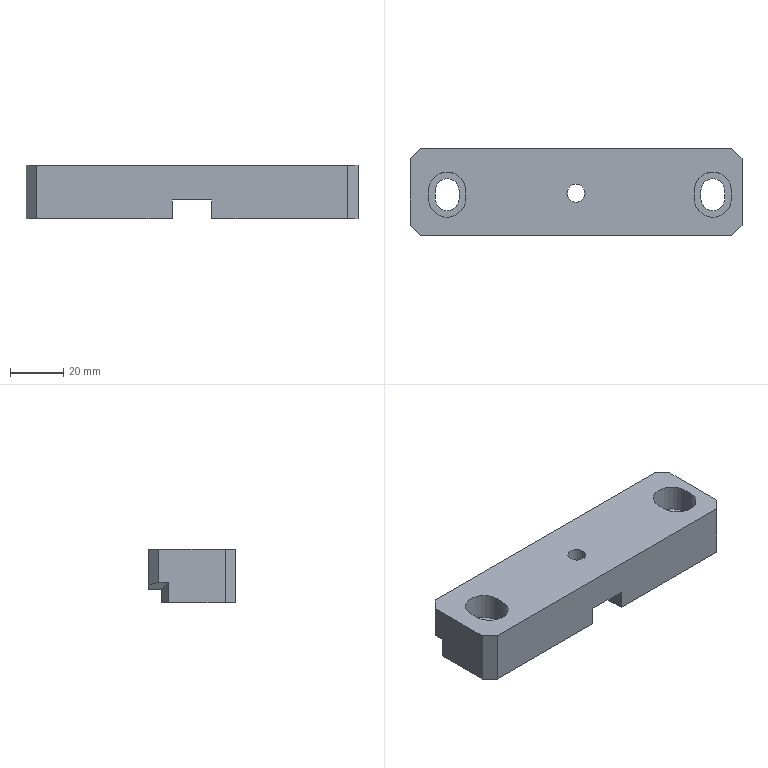Part | NX | features 20 2 | 1 solid | 41 faces | box 125 x 33 x 20 mm | volume 69243 mm3 | plane 32 | cylinder 9 | commonest cylinder face diameters 9 x4 14 x4 6.8 x1
STEP:
#1=CARTESIAN_POINT('',(3435.502,-433.5,16.5));
#2=VERTEX_POINT('',#1);
#3=CARTESIAN_POINT('',(3421.502,-433.5,16.5));
#4=VERTEX_POINT('',#3);
#5=CARTESIAN_POINT('',(3428.502,-433.5,16.5));
#6=DIRECTION('',(0.,0.,1.));
#7=DIRECTION('',(1.,0.,0.));
#8=AXIS2_PLACEMENT_3D('',#5,#6,#7);
#9=CIRCLE('',#8,7.);
#10=EDGE_CURVE('',#2,#4,#9,.T.);
#11=ORIENTED_EDGE('',*,*,#10,.F.);
#12=CARTESIAN_POINT('',(3435.502,-436.5,16.5));
#13=VERTEX_POINT('',#12);
#14=CARTESIAN_POINT('',(3435.502,-450.5,16.5));
#15=DIRECTION('',(0.,1.,0.));
#16=VECTOR('',#15,1000.);
#17=LINE('',#14,#16);
#18=EDGE_CURVE('',#13,#2,#17,.T.);
#19=ORIENTED_EDGE('',*,*,#18,.F.);
#20=CARTESIAN_POINT('',(3421.502,-436.5,16.5));
#21=VERTEX_POINT('',#20);
#22=CARTESIAN_POINT('',(3428.502,-436.5,16.5));
#23=DIRECTION('',(0.,0.,1.));
#24=DIRECTION('',(1.,0.,0.));
#25=AXIS2_PLACEMENT_3D('',#22,#23,#24);
#26=CIRCLE('',#25,7.);
#27=EDGE_CURVE('',#21,#13,#26,.T.);
#28=ORIENTED_EDGE('',*,*,#27,.F.);
#29=CARTESIAN_POINT('',(3421.502,-450.5,16.5));
#30=DIRECTION('',(0.,-1.,0.));
#31=VECTOR('',#30,1000.);
#32=LINE('',#29,#31);
#33=EDGE_CURVE('',#4,#21,#32,.T.);
#34=ORIENTED_EDGE('',*,*,#33,.F.);
#35=EDGE_LOOP('',(#11,#19,#28,#34));
#36=FACE_BOUND('',#35,.T.);
#37=CARTESIAN_POINT('',(3335.502,-436.5,16.5));
#38=VERTEX_POINT('',#37);
#39=CARTESIAN_POINT('',(3335.502,-433.5,16.5));
#40=VERTEX_POINT('',#39);
#41=CARTESIAN_POINT('',(3335.502,-450.5,16.5));
#42=DIRECTION('',(0.,1.,0.));
#43=VECTOR('',#42,1000.);
#44=LINE('',#41,#43);
#45=EDGE_CURVE('',#38,#40,#44,.T.);
#46=ORIENTED_EDGE('',*,*,#45,.F.);
#47=CARTESIAN_POINT('',(3321.502,-436.5,16.5));
#48=VERTEX_POINT('',#47);
#49=CARTESIAN_POINT('',(3328.502,-436.5,16.5));
#50=DIRECTION('',(0.,0.,1.));
#51=DIRECTION('',(1.,0.,0.));
#52=AXIS2_PLACEMENT_3D('',#49,#50,#51);
#53=CIRCLE('',#52,7.);
#54=EDGE_CURVE('',#48,#38,#53,.T.);
#55=ORIENTED_EDGE('',*,*,#54,.F.);
#56=CARTESIAN_POINT('',(3321.502,-433.5,16.5));
#57=VERTEX_POINT('',#56);
#58=CARTESIAN_POINT('',(3321.502,-450.5,16.5));
#59=DIRECTION('',(0.,-1.,0.));
#60=VECTOR('',#59,1000.);
#61=LINE('',#58,#60);
#62=EDGE_CURVE('',#57,#48,#61,.T.);
#63=ORIENTED_EDGE('',*,*,#62,.F.);
#64=CARTESIAN_POINT('',(3328.502,-433.5,16.5));
#65=DIRECTION('',(0.,0.,1.));
#66=DIRECTION('',(1.,0.,0.));
#67=AXIS2_PLACEMENT_3D('',#64,#65,#66);
#68=CIRCLE('',#67,7.);
#69=EDGE_CURVE('',#40,#57,#68,.T.);
#70=ORIENTED_EDGE('',*,*,#69,.F.);
#71=EDGE_LOOP('',(#46,#55,#63,#70));
#72=FACE_BOUND('',#71,.T.);
#73=CARTESIAN_POINT('',(3435.502,-417.5,16.5));
#74=VERTEX_POINT('',#73);
#75=CARTESIAN_POINT('',(3318.502,-417.5,16.5));
#76=VERTEX_POINT('',#75);
#77=CARTESIAN_POINT('',(3472.502,-417.5,16.5));
#78=DIRECTION('',(-1.,0.,0.));
#79=VECTOR('',#78,1000.);
#80=LINE('',#77,#79);
#81=EDGE_CURVE('',#74,#76,#80,.T.);
#82=ORIENTED_EDGE('',*,*,#81,.T.);
#83=CARTESIAN_POINT('',(3314.502,-421.5,16.5));
#84=VERTEX_POINT('',#83);
#85=CARTESIAN_POINT('',(3314.502,-421.5,16.5));
#86=DIRECTION('',(-0.7071,-0.7071,0.));
#87=VECTOR('',#86,1000.);
#88=LINE('',#85,#87);
#89=EDGE_CURVE('',#76,#84,#88,.T.);
#90=ORIENTED_EDGE('',*,*,#89,.T.);
#91=CARTESIAN_POINT('',(3314.502,-446.5,16.5));
#92=VERTEX_POINT('',#91);
#93=CARTESIAN_POINT('',(3314.502,-417.5,16.5));
#94=DIRECTION('',(0.,-1.,0.));
#95=VECTOR('',#94,1000.);
#96=LINE('',#93,#95);
#97=EDGE_CURVE('',#84,#92,#96,.T.);
#98=ORIENTED_EDGE('',*,*,#97,.T.);
#99=CARTESIAN_POINT('',(3318.502,-450.5,16.5));
#100=VERTEX_POINT('',#99);
#101=CARTESIAN_POINT('',(3318.502,-450.5,16.5));
#102=DIRECTION('',(0.7071,-0.7071,0.));
#103=VECTOR('',#102,1000.);
#104=LINE('',#101,#103);
#105=EDGE_CURVE('',#92,#100,#104,.T.);
#106=ORIENTED_EDGE('',*,*,#105,.T.);
#107=CARTESIAN_POINT('',(3435.502,-450.5,16.5));
#108=VERTEX_POINT('',#107);
#109=CARTESIAN_POINT('',(3392.502,-450.5,16.5));
#110=DIRECTION('',(1.,0.,0.));
#111=VECTOR('',#110,1000.);
#112=LINE('',#109,#111);
#113=EDGE_CURVE('',#100,#108,#112,.T.);
#114=ORIENTED_EDGE('',*,*,#113,.T.);
#115=CARTESIAN_POINT('',(3439.502,-446.5,16.5));
#116=VERTEX_POINT('',#115);
#117=CARTESIAN_POINT('',(3439.502,-446.5,16.5));
#118=DIRECTION('',(0.7071,0.7071,0.));
#119=VECTOR('',#118,1000.);
#120=LINE('',#117,#119);
#121=EDGE_CURVE('',#108,#116,#120,.T.);
#122=ORIENTED_EDGE('',*,*,#121,.T.);
#123=CARTESIAN_POINT('',(3439.502,-421.5,16.5));
#124=VERTEX_POINT('',#123);
#125=CARTESIAN_POINT('',(3439.502,-450.5,16.5));
#126=DIRECTION('',(0.,1.,0.));
#127=VECTOR('',#126,1000.);
#128=LINE('',#125,#127);
#129=EDGE_CURVE('',#116,#124,#128,.T.);
#130=ORIENTED_EDGE('',*,*,#129,.T.);
#131=CARTESIAN_POINT('',(3435.502,-417.5,16.5));
#132=DIRECTION('',(-0.7071,0.7071,0.));
#133=VECTOR('',#132,1000.);
#134=LINE('',#131,#133);
#135=EDGE_CURVE('',#124,#74,#134,.T.);
#136=ORIENTED_EDGE('',*,*,#135,.T.);
#137=EDGE_LOOP('',(#82,#90,#98,#106,#114,#122,#130,#136));
#138=FACE_BOUND('',#137,.T.);
#139=CARTESIAN_POINT('',(3380.402,-434.5,16.5));
#140=VERTEX_POINT('',#139);
#141=CARTESIAN_POINT('',(3377.002,-434.5,16.5));
#142=DIRECTION('',(0.,0.,-1.));
#143=DIRECTION('',(1.,0.,0.));
#144=AXIS2_PLACEMENT_3D('',#141,#142,#143);
#145=CIRCLE('',#144,3.4);
#146=EDGE_CURVE('',#140,#140,#145,.T.);
#147=ORIENTED_EDGE('',*,*,#146,.T.);
#148=EDGE_LOOP('',(#147));
#149=FACE_BOUND('',#148,.T.);
#150=CARTESIAN_POINT('',(3472.502,-450.5,16.5));
#151=DIRECTION('',(0.,0.,1.));
#152=DIRECTION('',(-1.,0.,0.));
#153=AXIS2_PLACEMENT_3D('',#150,#151,#152);
#154=PLANE('',#153);
#155=ADVANCED_FACE('',(#36,#72,#138,#149),#154,.T.);
#156=CARTESIAN_POINT('',(3384.502,-417.5,3.5));
#157=VERTEX_POINT('',#156);
#158=CARTESIAN_POINT('',(3384.502,-450.5,3.5));
#159=VERTEX_POINT('',#158);
#160=CARTESIAN_POINT('',(3384.502,-436.5,3.5));
#161=DIRECTION('',(0.,-1.,0.));
#162=VECTOR('',#161,1000.);
#163=LINE('',#160,#162);
#164=EDGE_CURVE('',#157,#159,#163,.T.);
#165=ORIENTED_EDGE('',*,*,#164,.F.);
#166=CARTESIAN_POINT('',(3384.502,-417.5,1.5));
#167=VERTEX_POINT('',#166);
#168=CARTESIAN_POINT('',(3384.502,-417.5,11.5));
#169=DIRECTION('',(0.,0.,-1.));
#170=VECTOR('',#169,1000.);
#171=LINE('',#168,#170);
#172=EDGE_CURVE('',#157,#167,#171,.T.);
#173=ORIENTED_EDGE('',*,*,#172,.T.);
#174=CARTESIAN_POINT('',(3384.502,-422.5,1.5));
#175=VERTEX_POINT('',#174);
#176=CARTESIAN_POINT('',(3384.502,-396.891,1.5));
#177=DIRECTION('',(0.,1.,0.));
#178=VECTOR('',#177,1000.);
#179=LINE('',#176,#178);
#180=EDGE_CURVE('',#175,#167,#179,.T.);
#181=ORIENTED_EDGE('',*,*,#180,.F.);
#182=CARTESIAN_POINT('',(3384.502,-422.5,-3.5));
#183=VERTEX_POINT('',#182);
#184=CARTESIAN_POINT('',(3384.502,-422.5,3.5));
#185=DIRECTION('',(0.,0.,-1.));
#186=VECTOR('',#185,1000.);
#187=LINE('',#184,#186);
#188=EDGE_CURVE('',#175,#183,#187,.T.);
#189=ORIENTED_EDGE('',*,*,#188,.T.);
#190=CARTESIAN_POINT('',(3384.502,-450.5,-3.5));
#191=VERTEX_POINT('',#190);
#192=CARTESIAN_POINT('',(3384.502,-450.5,-3.5));
#193=DIRECTION('',(0.,-1.,0.));
#194=VECTOR('',#193,1000.);
#195=LINE('',#192,#194);
#196=EDGE_CURVE('',#183,#191,#195,.T.);
#197=ORIENTED_EDGE('',*,*,#196,.T.);
#198=CARTESIAN_POINT('',(3384.502,-450.5,11.5));
#199=DIRECTION('',(0.,0.,1.));
#200=VECTOR('',#199,1000.);
#201=LINE('',#198,#200);
#202=EDGE_CURVE('',#191,#159,#201,.T.);
#203=ORIENTED_EDGE('',*,*,#202,.T.);
#204=EDGE_LOOP('',(#165,#173,#181,#189,#197,#203));
#205=FACE_BOUND('',#204,.T.);
#206=CARTESIAN_POINT('',(3384.502,-436.5,0.));
#207=DIRECTION('',(-1.,0.,0.));
#208=DIRECTION('',(0.,0.,1.));
#209=AXIS2_PLACEMENT_3D('',#206,#207,#208);
#210=PLANE('',#209);
#211=ADVANCED_FACE('',(#205),#210,.T.);
#212=CARTESIAN_POINT('',(3369.502,-422.5,-3.5));
#213=VERTEX_POINT('',#212);
#214=CARTESIAN_POINT('',(3369.502,-450.5,-3.5));
#215=VERTEX_POINT('',#214);
#216=CARTESIAN_POINT('',(3369.502,-450.5,-3.5));
#217=DIRECTION('',(0.,-1.,0.));
#218=VECTOR('',#217,1000.);
#219=LINE('',#216,#218);
#220=EDGE_CURVE('',#213,#215,#219,.T.);
#221=ORIENTED_EDGE('',*,*,#220,.F.);
#222=CARTESIAN_POINT('',(3369.502,-422.5,1.5));
#223=VERTEX_POINT('',#222);
#224=CARTESIAN_POINT('',(3369.502,-422.5,3.5));
#225=DIRECTION('',(0.,0.,-1.));
#226=VECTOR('',#225,1000.);
#227=LINE('',#224,#226);
#228=EDGE_CURVE('',#223,#213,#227,.T.);
#229=ORIENTED_EDGE('',*,*,#228,.F.);
#230=CARTESIAN_POINT('',(3369.502,-417.5,1.5));
#231=VERTEX_POINT('',#230);
#232=CARTESIAN_POINT('',(3369.502,-396.891,1.5));
#233=DIRECTION('',(0.,1.,0.));
#234=VECTOR('',#233,1000.);
#235=LINE('',#232,#234);
#236=EDGE_CURVE('',#223,#231,#235,.T.);
#237=ORIENTED_EDGE('',*,*,#236,.T.);
#238=CARTESIAN_POINT('',(3369.502,-417.5,3.5));
#239=VERTEX_POINT('',#238);
#240=CARTESIAN_POINT('',(3369.502,-417.5,11.5));
#241=DIRECTION('',(0.,0.,-1.));
#242=VECTOR('',#241,1000.);
#243=LINE('',#240,#242);
#244=EDGE_CURVE('',#239,#231,#243,.T.);
#245=ORIENTED_EDGE('',*,*,#244,.F.);
#246=CARTESIAN_POINT('',(3369.502,-450.5,3.5));
#247=VERTEX_POINT('',#246);
#248=CARTESIAN_POINT('',(3369.502,-436.5,3.5));
#249=DIRECTION('',(0.,1.,0.));
#250=VECTOR('',#249,1000.);
#251=LINE('',#248,#250);
#252=EDGE_CURVE('',#247,#239,#251,.T.);
#253=ORIENTED_EDGE('',*,*,#252,.F.);
#254=CARTESIAN_POINT('',(3369.502,-450.5,11.5));
#255=DIRECTION('',(0.,0.,1.));
#256=VECTOR('',#255,1000.);
#257=LINE('',#254,#256);
#258=EDGE_CURVE('',#215,#247,#257,.T.);
#259=ORIENTED_EDGE('',*,*,#258,.F.);
#260=EDGE_LOOP('',(#221,#229,#237,#245,#253,#259));
#261=FACE_BOUND('',#260,.T.);
#262=CARTESIAN_POINT('',(3369.502,-436.5,-9.5));
#263=DIRECTION('',(-1.,0.,0.));
#264=DIRECTION('',(0.,0.,-1.));
#265=AXIS2_PLACEMENT_3D('',#262,#263,#264);
#266=PLANE('',#265);
#267=ADVANCED_FACE('',(#261),#266,.F.);
#268=CARTESIAN_POINT('',(3380.402,-434.5,3.5));
#269=VERTEX_POINT('',#268);
#270=CARTESIAN_POINT('',(3377.002,-434.5,3.5));
#271=DIRECTION('',(0.,0.,1.));
#272=DIRECTION('',(1.,0.,0.));
#273=AXIS2_PLACEMENT_3D('',#270,#271,#272);
#274=CIRCLE('',#273,3.4);
#275=EDGE_CURVE('',#269,#269,#274,.T.);
#276=ORIENTED_EDGE('',*,*,#275,.T.);
#277=EDGE_LOOP('',(#276));
#278=FACE_BOUND('',#277,.T.);
#279=CARTESIAN_POINT('',(3447.502,-450.5,3.5));
#280=DIRECTION('',(1.,0.,0.));
#281=VECTOR('',#280,1000.);
#282=LINE('',#279,#281);
#283=EDGE_CURVE('',#247,#159,#282,.T.);
#284=ORIENTED_EDGE('',*,*,#283,.F.);
#285=ORIENTED_EDGE('',*,*,#252,.T.);
#286=CARTESIAN_POINT('',(3527.502,-417.5,3.5));
#287=DIRECTION('',(-1.,0.,0.));
#288=VECTOR('',#287,1000.);
#289=LINE('',#286,#288);
#290=EDGE_CURVE('',#157,#239,#289,.T.);
#291=ORIENTED_EDGE('',*,*,#290,.F.);
#292=ORIENTED_EDGE('',*,*,#164,.T.);
#293=EDGE_LOOP('',(#284,#285,#291,#292));
#294=FACE_BOUND('',#293,.T.);
#295=CARTESIAN_POINT('',(3377.002,-436.5,3.5));
#296=DIRECTION('',(0.,0.,1.));
#297=DIRECTION('',(0.,-1.,0.));
#298=AXIS2_PLACEMENT_3D('',#295,#296,#297);
#299=PLANE('',#298);
#300=ADVANCED_FACE('',(#278,#294),#299,.F.);
#301=CARTESIAN_POINT('',(3424.002,-436.5,6.5));
#302=VERTEX_POINT('',#301);
#303=CARTESIAN_POINT('',(3424.002,-433.5,6.5));
#304=VERTEX_POINT('',#303);
#305=CARTESIAN_POINT('',(3424.002,-432.5,6.5));
#306=DIRECTION('',(0.,1.,0.));
#307=VECTOR('',#306,1000.);
#308=LINE('',#305,#307);
#309=EDGE_CURVE('',#302,#304,#308,.T.);
#310=ORIENTED_EDGE('',*,*,#309,.T.);
#311=CARTESIAN_POINT('',(3433.002,-433.5,6.5));
#312=VERTEX_POINT('',#311);
#313=CARTESIAN_POINT('',(3428.502,-433.5,6.5));
#314=DIRECTION('',(0.,0.,-1.));
#315=DIRECTION('',(-1.,0.,0.));
#316=AXIS2_PLACEMENT_3D('',#313,#314,#315);
#317=CIRCLE('',#316,4.5);
#318=EDGE_CURVE('',#304,#312,#317,.T.);
#319=ORIENTED_EDGE('',*,*,#318,.T.);
#320=CARTESIAN_POINT('',(3433.002,-436.5,6.5));
#321=VERTEX_POINT('',#320);
#322=CARTESIAN_POINT('',(3433.002,-439.5,6.5));
#323=DIRECTION('',(0.,-1.,0.));
#324=VECTOR('',#323,1000.);
#325=LINE('',#322,#324);
#326=EDGE_CURVE('',#312,#321,#325,.T.);
#327=ORIENTED_EDGE('',*,*,#326,.T.);
#328=CARTESIAN_POINT('',(3428.502,-436.5,6.5));
#329=DIRECTION('',(0.,0.,-1.));
#330=DIRECTION('',(-1.,0.,0.));
#331=AXIS2_PLACEMENT_3D('',#328,#329,#330);
#332=CIRCLE('',#331,4.5);
#333=EDGE_CURVE('',#321,#302,#332,.T.);
#334=ORIENTED_EDGE('',*,*,#333,.T.);
#335=EDGE_LOOP('',(#310,#319,#327,#334));
#336=FACE_BOUND('',#335,.T.);
#337=CARTESIAN_POINT('',(3435.502,-433.5,6.5));
#338=VERTEX_POINT('',#337);
#339=CARTESIAN_POINT('',(3421.502,-433.5,6.5));
#340=VERTEX_POINT('',#339);
#341=CARTESIAN_POINT('',(3428.502,-433.5,6.5));
#342=DIRECTION('',(0.,0.,1.));
#343=DIRECTION('',(-1.,0.,0.));
#344=AXIS2_PLACEMENT_3D('',#341,#342,#343);
#345=CIRCLE('',#344,7.);
#346=EDGE_CURVE('',#338,#340,#345,.T.);
#347=ORIENTED_EDGE('',*,*,#346,.T.);
#348=CARTESIAN_POINT('',(3421.502,-436.5,6.5));
#349=VERTEX_POINT('',#348);
#350=CARTESIAN_POINT('',(3421.502,-439.5,6.5));
#351=DIRECTION('',(0.,-1.,0.));
#352=VECTOR('',#351,1000.);
#353=LINE('',#350,#352);
#354=EDGE_CURVE('',#340,#349,#353,.T.);
#355=ORIENTED_EDGE('',*,*,#354,.T.);
#356=CARTESIAN_POINT('',(3435.502,-436.5,6.5));
#357=VERTEX_POINT('',#356);
#358=CARTESIAN_POINT('',(3428.502,-436.5,6.5));
#359=DIRECTION('',(0.,0.,1.));
#360=DIRECTION('',(-1.,0.,0.));
#361=AXIS2_PLACEMENT_3D('',#358,#359,#360);
#362=CIRCLE('',#361,7.);
#363=EDGE_CURVE('',#349,#357,#362,.T.);
#364=ORIENTED_EDGE('',*,*,#363,.T.);
#365=CARTESIAN_POINT('',(3435.502,-432.5,6.5));
#366=DIRECTION('',(0.,1.,0.));
#367=VECTOR('',#366,1000.);
#368=LINE('',#365,#367);
#369=EDGE_CURVE('',#357,#338,#368,.T.);
#370=ORIENTED_EDGE('',*,*,#369,.T.);
#371=EDGE_LOOP('',(#347,#355,#364,#370));
#372=FACE_BOUND('',#371,.T.);
#373=CARTESIAN_POINT('',(3428.502,-432.5,6.5));
#374=DIRECTION('',(0.,0.,-1.));
#375=DIRECTION('',(1.,0.,0.));
#376=AXIS2_PLACEMENT_3D('',#373,#374,#375);
#377=PLANE('',#376);
#378=ADVANCED_FACE('',(#336,#372),#377,.F.);
#379=CARTESIAN_POINT('',(3429.502,-417.5,1.5));
#380=VERTEX_POINT('',#379);
#381=CARTESIAN_POINT('',(3429.502,-422.5,1.5));
#382=VERTEX_POINT('',#381);
#383=CARTESIAN_POINT('',(3429.502,-425.18,1.5));
#384=DIRECTION('',(0.,-1.,0.));
#385=VECTOR('',#384,1000.);
#386=LINE('',#383,#385);
#387=EDGE_CURVE('',#380,#382,#386,.T.);
#388=ORIENTED_EDGE('',*,*,#387,.F.);
#389=CARTESIAN_POINT('',(3435.502,-417.5,3.108));
#390=VERTEX_POINT('',#389);
#391=CARTESIAN_POINT('',(3429.502,-417.5,1.5));
#392=DIRECTION('',(-0.9659,0.,-0.2588));
#393=VECTOR('',#392,1000.);
#394=LINE('',#391,#393);
#395=EDGE_CURVE('',#390,#380,#394,.T.);
#396=ORIENTED_EDGE('',*,*,#395,.F.);
#397=CARTESIAN_POINT('',(3439.502,-421.5,4.179));
#398=VERTEX_POINT('',#397);
#399=CARTESIAN_POINT('',(3422.451,-404.449,-0.3894));
#400=DIRECTION('',(0.6947,-0.6947,0.1862));
#401=VECTOR('',#400,1000.);
#402=LINE('',#399,#401);
#403=EDGE_CURVE('',#390,#398,#402,.T.);
#404=ORIENTED_EDGE('',*,*,#403,.T.);
#405=CARTESIAN_POINT('',(3439.502,-425.18,4.179));
#406=VERTEX_POINT('',#405);
#407=CARTESIAN_POINT('',(3439.502,-417.5,4.179));
#408=DIRECTION('',(0.,1.,0.));
#409=VECTOR('',#408,1000.);
#410=LINE('',#407,#409);
#411=EDGE_CURVE('',#406,#398,#410,.T.);
#412=ORIENTED_EDGE('',*,*,#411,.F.);
#413=CARTESIAN_POINT('',(3438.875,-425.012,4.011));
#414=DIRECTION('',(0.9351,-0.2506,0.2506));
#415=VECTOR('',#414,1000.);
#416=LINE('',#413,#415);
#417=EDGE_CURVE('',#382,#406,#416,.T.);
#418=ORIENTED_EDGE('',*,*,#417,.F.);
#419=EDGE_LOOP('',(#388,#396,#404,#412,#418));
#420=FACE_BOUND('',#419,.T.);
#421=CARTESIAN_POINT('',(3429.502,-396.891,1.5));
#422=DIRECTION('',(0.2588,0.,-0.9659));
#423=DIRECTION('',(0.9659,0.,0.2588));
#424=AXIS2_PLACEMENT_3D('',#421,#422,#423);
#425=PLANE('',#424);
#426=ADVANCED_FACE('',(#420),#425,.T.);
#427=CARTESIAN_POINT('',(3333.002,-433.5,6.5));
#428=VERTEX_POINT('',#427);
#429=CARTESIAN_POINT('',(3333.002,-436.5,6.5));
#430=VERTEX_POINT('',#429);
#431=CARTESIAN_POINT('',(3333.002,-432.5,6.5));
#432=DIRECTION('',(0.,-1.,0.));
#433=VECTOR('',#432,1000.);
#434=LINE('',#431,#433);
#435=EDGE_CURVE('',#428,#430,#434,.T.);
#436=ORIENTED_EDGE('',*,*,#435,.T.);
#437=CARTESIAN_POINT('',(3324.002,-436.5,6.5));
#438=VERTEX_POINT('',#437);
#439=CARTESIAN_POINT('',(3328.502,-436.5,6.5));
#440=DIRECTION('',(0.,0.,-1.));
#441=DIRECTION('',(-1.,0.,0.));
#442=AXIS2_PLACEMENT_3D('',#439,#440,#441);
#443=CIRCLE('',#442,4.5);
#444=EDGE_CURVE('',#430,#438,#443,.T.);
#445=ORIENTED_EDGE('',*,*,#444,.T.);
#446=CARTESIAN_POINT('',(3324.002,-433.5,6.5));
#447=VERTEX_POINT('',#446);
#448=CARTESIAN_POINT('',(3324.002,-439.5,6.5));
#449=DIRECTION('',(0.,1.,0.));
#450=VECTOR('',#449,1000.);
#451=LINE('',#448,#450);
#452=EDGE_CURVE('',#438,#447,#451,.T.);
#453=ORIENTED_EDGE('',*,*,#452,.T.);
#454=CARTESIAN_POINT('',(3328.502,-433.5,6.5));
#455=DIRECTION('',(0.,0.,-1.));
#456=DIRECTION('',(-1.,0.,0.));
#457=AXIS2_PLACEMENT_3D('',#454,#455,#456);
#458=CIRCLE('',#457,4.5);
#459=EDGE_CURVE('',#447,#428,#458,.T.);
#460=ORIENTED_EDGE('',*,*,#459,.T.);
#461=EDGE_LOOP('',(#436,#445,#453,#460));
#462=FACE_BOUND('',#461,.T.);
#463=CARTESIAN_POINT('',(3335.502,-433.5,6.5));
#464=VERTEX_POINT('',#463);
#465=CARTESIAN_POINT('',(3321.502,-433.5,6.5));
#466=VERTEX_POINT('',#465);
#467=CARTESIAN_POINT('',(3328.502,-433.5,6.5));
#468=DIRECTION('',(0.,0.,1.));
#469=DIRECTION('',(-1.,0.,0.));
#470=AXIS2_PLACEMENT_3D('',#467,#468,#469);
#471=CIRCLE('',#470,7.);
#472=EDGE_CURVE('',#464,#466,#471,.T.);
#473=ORIENTED_EDGE('',*,*,#472,.T.);
#474=CARTESIAN_POINT('',(3321.502,-436.5,6.5));
#475=VERTEX_POINT('',#474);
#476=CARTESIAN_POINT('',(3321.502,-432.5,6.5));
#477=DIRECTION('',(0.,-1.,0.));
#478=VECTOR('',#477,1000.);
#479=LINE('',#476,#478);
#480=EDGE_CURVE('',#466,#475,#479,.T.);
#481=ORIENTED_EDGE('',*,*,#480,.T.);
#482=CARTESIAN_POINT('',(3335.502,-436.5,6.5));
#483=VERTEX_POINT('',#482);
#484=CARTESIAN_POINT('',(3328.502,-436.5,6.5));
#485=DIRECTION('',(0.,0.,1.));
#486=DIRECTION('',(-1.,0.,0.));
#487=AXIS2_PLACEMENT_3D('',#484,#485,#486);
#488=CIRCLE('',#487,7.);
#489=EDGE_CURVE('',#475,#483,#488,.T.);
#490=ORIENTED_EDGE('',*,*,#489,.T.);
#491=CARTESIAN_POINT('',(3335.502,-439.5,6.5));
#492=DIRECTION('',(0.,1.,0.));
#493=VECTOR('',#492,1000.);
#494=LINE('',#491,#493);
#495=EDGE_CURVE('',#483,#464,#494,.T.);
#496=ORIENTED_EDGE('',*,*,#495,.T.);
#497=EDGE_LOOP('',(#473,#481,#490,#496));
#498=FACE_BOUND('',#497,.T.);
#499=CARTESIAN_POINT('',(3328.502,-432.5,6.5));
#500=DIRECTION('',(0.,0.,-1.));
#501=DIRECTION('',(-1.,0.,0.));
#502=AXIS2_PLACEMENT_3D('',#499,#500,#501);
#503=PLANE('',#502);
#504=ADVANCED_FACE('',(#462,#498),#503,.F.);
#505=ORIENTED_EDGE('',*,*,#33,.T.);
#506=CARTESIAN_POINT('',(3421.502,-436.5,42.5));
#507=DIRECTION('',(0.,0.,1.));
#508=VECTOR('',#507,1000.);
#509=LINE('',#506,#508);
#510=EDGE_CURVE('',#349,#21,#509,.T.);
#511=ORIENTED_EDGE('',*,*,#510,.F.);
#512=ORIENTED_EDGE('',*,*,#354,.F.);
#513=CARTESIAN_POINT('',(3421.502,-433.5,42.5));
#514=DIRECTION('',(0.,0.,1.));
#515=VECTOR('',#514,1000.);
#516=LINE('',#513,#515);
#517=EDGE_CURVE('',#340,#4,#516,.T.);
#518=ORIENTED_EDGE('',*,*,#517,.T.);
#519=EDGE_LOOP('',(#505,#511,#512,#518));
#520=FACE_BOUND('',#519,.T.);
#521=CARTESIAN_POINT('',(3421.502,-439.5,42.5));
#522=DIRECTION('',(-1.,0.,0.));
#523=DIRECTION('',(0.,0.,-1.));
#524=AXIS2_PLACEMENT_3D('',#521,#522,#523);
#525=PLANE('',#524);
#526=ADVANCED_FACE('',(#520),#525,.F.);
#527=ORIENTED_EDGE('',*,*,#27,.T.);
#528=CARTESIAN_POINT('',(3435.502,-436.5,42.5));
#529=DIRECTION('',(0.,0.,1.));
#530=VECTOR('',#529,1000.);
#531=LINE('',#528,#530);
#532=EDGE_CURVE('',#357,#13,#531,.T.);
#533=ORIENTED_EDGE('',*,*,#532,.F.);
#534=ORIENTED_EDGE('',*,*,#363,.F.);
#535=ORIENTED_EDGE('',*,*,#510,.T.);
#536=EDGE_LOOP('',(#527,#533,#534,#535));
#537=FACE_BOUND('',#536,.T.);
#538=CARTESIAN_POINT('',(3428.502,-436.5,42.5));
#539=DIRECTION('',(0.,0.,-1.));
#540=DIRECTION('',(1.,0.,0.));
#541=AXIS2_PLACEMENT_3D('',#538,#539,#540);
#542=CYLINDRICAL_SURFACE('',#541,7.);
#543=ADVANCED_FACE('',(#537),#542,.F.);
#544=ORIENTED_EDGE('',*,*,#18,.T.);
#545=CARTESIAN_POINT('',(3435.502,-433.5,42.5));
#546=DIRECTION('',(0.,0.,1.));
#547=VECTOR('',#546,1000.);
#548=LINE('',#545,#547);
#549=EDGE_CURVE('',#338,#2,#548,.T.);
#550=ORIENTED_EDGE('',*,*,#549,.F.);
#551=ORIENTED_EDGE('',*,*,#369,.F.);
#552=ORIENTED_EDGE('',*,*,#532,.T.);
#553=EDGE_LOOP('',(#544,#550,#551,#552));
#554=FACE_BOUND('',#553,.T.);
#555=CARTESIAN_POINT('',(3435.502,-432.5,42.5));
#556=DIRECTION('',(1.,0.,0.));
#557=DIRECTION('',(0.,0.,1.));
#558=AXIS2_PLACEMENT_3D('',#555,#556,#557);
#559=PLANE('',#558);
#560=ADVANCED_FACE('',(#554),#559,.F.);
#561=ORIENTED_EDGE('',*,*,#10,.T.);
#562=ORIENTED_EDGE('',*,*,#517,.F.);
#563=ORIENTED_EDGE('',*,*,#346,.F.);
#564=ORIENTED_EDGE('',*,*,#549,.T.);
#565=EDGE_LOOP('',(#561,#562,#563,#564));
#566=FACE_BOUND('',#565,.T.);
#567=CARTESIAN_POINT('',(3428.502,-433.5,42.5));
#568=DIRECTION('',(0.,0.,-1.));
#569=DIRECTION('',(1.,0.,0.));
#570=AXIS2_PLACEMENT_3D('',#567,#568,#569);
#571=CYLINDRICAL_SURFACE('',#570,7.);
#572=ADVANCED_FACE('',(#566),#571,.F.);
#573=ORIENTED_EDGE('',*,*,#135,.F.);
#574=CARTESIAN_POINT('',(3439.502,-421.5,11.5));
#575=DIRECTION('',(0.,0.,1.));
#576=VECTOR('',#575,1000.);
#577=LINE('',#574,#576);
#578=EDGE_CURVE('',#398,#124,#577,.T.);
#579=ORIENTED_EDGE('',*,*,#578,.F.);
#580=ORIENTED_EDGE('',*,*,#403,.F.);
#581=CARTESIAN_POINT('',(3435.502,-417.5,11.5));
#582=DIRECTION('',(0.,0.,-1.));
#583=VECTOR('',#582,1000.);
#584=LINE('',#581,#583);
#585=EDGE_CURVE('',#74,#390,#584,.T.);
#586=ORIENTED_EDGE('',*,*,#585,.F.);
#587=EDGE_LOOP('',(#573,#579,#580,#586));
#588=FACE_BOUND('',#587,.T.);
#589=CARTESIAN_POINT('',(3435.502,-417.5,11.5));
#590=DIRECTION('',(-0.7071,-0.7071,0.));
#591=DIRECTION('',(0.,0.,-1.));
#592=AXIS2_PLACEMENT_3D('',#589,#590,#591);
#593=PLANE('',#592);
#594=ADVANCED_FACE('',(#588),#593,.F.);
#595=ORIENTED_EDGE('',*,*,#69,.T.);
#596=CARTESIAN_POINT('',(3321.502,-433.5,42.5));
#597=DIRECTION('',(0.,0.,-1.));
#598=VECTOR('',#597,1000.);
#599=LINE('',#596,#598);
#600=EDGE_CURVE('',#57,#466,#599,.T.);
#601=ORIENTED_EDGE('',*,*,#600,.T.);
#602=ORIENTED_EDGE('',*,*,#472,.F.);
#603=CARTESIAN_POINT('',(3335.502,-433.5,42.5));
#604=DIRECTION('',(0.,0.,-1.));
#605=VECTOR('',#604,1000.);
#606=LINE('',#603,#605);
#607=EDGE_CURVE('',#40,#464,#606,.T.);
#608=ORIENTED_EDGE('',*,*,#607,.F.);
#609=EDGE_LOOP('',(#595,#601,#602,#608));
#610=FACE_BOUND('',#609,.T.);
#611=CARTESIAN_POINT('',(3328.502,-433.5,42.5));
#612=DIRECTION('',(0.,0.,-1.));
#613=DIRECTION('',(-1.,0.,0.));
#614=AXIS2_PLACEMENT_3D('',#611,#612,#613);
#615=CYLINDRICAL_SURFACE('',#614,7.);
#616=ADVANCED_FACE('',(#610),#615,.F.);
#617=ORIENTED_EDGE('',*,*,#62,.T.);
#618=CARTESIAN_POINT('',(3321.502,-436.5,42.5));
#619=DIRECTION('',(0.,0.,-1.));
#620=VECTOR('',#619,1000.);
#621=LINE('',#618,#620);
#622=EDGE_CURVE('',#48,#475,#621,.T.);
#623=ORIENTED_EDGE('',*,*,#622,.T.);
#624=ORIENTED_EDGE('',*,*,#480,.F.);
#625=ORIENTED_EDGE('',*,*,#600,.F.);
#626=EDGE_LOOP('',(#617,#623,#624,#625));
#627=FACE_BOUND('',#626,.T.);
#628=CARTESIAN_POINT('',(3321.502,-432.5,42.5));
#629=DIRECTION('',(-1.,0.,0.));
#630=DIRECTION('',(0.,0.,1.));
#631=AXIS2_PLACEMENT_3D('',#628,#629,#630);
#632=PLANE('',#631);
#633=ADVANCED_FACE('',(#627),#632,.F.);
#634=ORIENTED_EDGE('',*,*,#54,.T.);
#635=CARTESIAN_POINT('',(3335.502,-436.5,42.5));
#636=DIRECTION('',(0.,0.,-1.));
#637=VECTOR('',#636,1000.);
#638=LINE('',#635,#637);
#639=EDGE_CURVE('',#38,#483,#638,.T.);
#640=ORIENTED_EDGE('',*,*,#639,.T.);
#641=ORIENTED_EDGE('',*,*,#489,.F.);
#642=ORIENTED_EDGE('',*,*,#622,.F.);
#643=EDGE_LOOP('',(#634,#640,#641,#642));
#644=FACE_BOUND('',#643,.T.);
#645=CARTESIAN_POINT('',(3328.502,-436.5,42.5));
#646=DIRECTION('',(0.,0.,-1.));
#647=DIRECTION('',(-1.,0.,0.));
#648=AXIS2_PLACEMENT_3D('',#645,#646,#647);
#649=CYLINDRICAL_SURFACE('',#648,7.);
#650=ADVANCED_FACE('',(#644),#649,.F.);
#651=ORIENTED_EDGE('',*,*,#45,.T.);
#652=ORIENTED_EDGE('',*,*,#607,.T.);
#653=ORIENTED_EDGE('',*,*,#495,.F.);
#654=ORIENTED_EDGE('',*,*,#639,.F.);
#655=EDGE_LOOP('',(#651,#652,#653,#654));
#656=FACE_BOUND('',#655,.T.);
#657=CARTESIAN_POINT('',(3335.502,-439.5,42.5));
#658=DIRECTION('',(1.,0.,0.));
#659=DIRECTION('',(0.,0.,-1.));
#660=AXIS2_PLACEMENT_3D('',#657,#658,#659);
#661=PLANE('',#660);
#662=ADVANCED_FACE('',(#656),#661,.F.);
#663=ORIENTED_EDGE('',*,*,#411,.T.);
#664=ORIENTED_EDGE('',*,*,#578,.T.);
#665=ORIENTED_EDGE('',*,*,#129,.F.);
#666=CARTESIAN_POINT('',(3439.502,-446.5,-3.5));
#667=VERTEX_POINT('',#666);
#668=CARTESIAN_POINT('',(3439.502,-446.5,11.5));
#669=DIRECTION('',(0.,0.,-1.));
#670=VECTOR('',#669,1000.);
#671=LINE('',#668,#670);
#672=EDGE_CURVE('',#116,#667,#671,.T.);
#673=ORIENTED_EDGE('',*,*,#672,.T.);
#674=CARTESIAN_POINT('',(3439.502,-425.18,-3.5));
#675=VERTEX_POINT('',#674);
#676=CARTESIAN_POINT('',(3439.502,-450.5,-3.5));
#677=DIRECTION('',(0.,1.,0.));
#678=VECTOR('',#677,1000.);
#679=LINE('',#676,#678);
#680=EDGE_CURVE('',#667,#675,#679,.T.);
#681=ORIENTED_EDGE('',*,*,#680,.T.);
#682=CARTESIAN_POINT('',(3439.502,-425.18,3.5));
#683=DIRECTION('',(0.,0.,-1.));
#684=VECTOR('',#683,1000.);
#685=LINE('',#682,#684);
#686=EDGE_CURVE('',#406,#675,#685,.T.);
#687=ORIENTED_EDGE('',*,*,#686,.F.);
#688=EDGE_LOOP('',(#663,#664,#665,#673,#681,#687));
#689=FACE_BOUND('',#688,.T.);
#690=CARTESIAN_POINT('',(3439.502,-450.5,11.5));
#691=DIRECTION('',(-1.,0.,0.));
#692=DIRECTION('',(0.,0.,-1.));
#693=AXIS2_PLACEMENT_3D('',#690,#691,#692);
#694=PLANE('',#693);
#695=ADVANCED_FACE('',(#689),#694,.F.);
#696=CARTESIAN_POINT('',(3429.501,-422.5,1.5));
#697=VERTEX_POINT('',#696);
#698=CARTESIAN_POINT('',(3439.502,-425.18,1.5));
#699=DIRECTION('',(0.9659,-0.2588,0.));
#700=VECTOR('',#699,1000.);
#701=LINE('',#698,#700);
#702=EDGE_CURVE('',#697,#382,#701,.T.);
#703=ORIENTED_EDGE('',*,*,#702,.T.);
#704=ORIENTED_EDGE('',*,*,#417,.T.);
#705=ORIENTED_EDGE('',*,*,#686,.T.);
#706=CARTESIAN_POINT('',(3429.501,-422.5,-3.5));
#707=VERTEX_POINT('',#706);
#708=CARTESIAN_POINT('',(3439.502,-425.18,-3.5));
#709=DIRECTION('',(-0.9659,0.2588,0.));
#710=VECTOR('',#709,1000.);
#711=LINE('',#708,#710);
#712=EDGE_CURVE('',#675,#707,#711,.T.);
#713=ORIENTED_EDGE('',*,*,#712,.T.);
#714=CARTESIAN_POINT('',(3429.501,-422.5,3.5));
#715=DIRECTION('',(0.,0.,1.));
#716=VECTOR('',#715,1000.);
#717=LINE('',#714,#716);
#718=EDGE_CURVE('',#707,#697,#717,.T.);
#719=ORIENTED_EDGE('',*,*,#718,.T.);
#720=EDGE_LOOP('',(#703,#704,#705,#713,#719));
#721=FACE_BOUND('',#720,.T.);
#722=CARTESIAN_POINT('',(3439.502,-425.18,3.5));
#723=DIRECTION('',(-0.2588,-0.9659,0.));
#724=DIRECTION('',(0.9659,-0.2588,0.));
#725=AXIS2_PLACEMENT_3D('',#722,#723,#724);
#726=PLANE('',#725);
#727=ADVANCED_FACE('',(#721),#726,.F.);
#728=ORIENTED_EDGE('',*,*,#318,.F.);
#729=CARTESIAN_POINT('',(3424.002,-433.5,-3.5));
#730=VERTEX_POINT('',#729);
#731=CARTESIAN_POINT('',(3424.002,-433.5,42.5));
#732=DIRECTION('',(0.,0.,1.));
#733=VECTOR('',#732,1000.);
#734=LINE('',#731,#733);
#735=EDGE_CURVE('',#730,#304,#734,.T.);
#736=ORIENTED_EDGE('',*,*,#735,.F.);
#737=CARTESIAN_POINT('',(3433.002,-433.5,-3.5));
#738=VERTEX_POINT('',#737);
#739=CARTESIAN_POINT('',(3428.502,-433.5,-3.5));
#740=DIRECTION('',(0.,0.,1.));
#741=DIRECTION('',(1.,0.,0.));
#742=AXIS2_PLACEMENT_3D('',#739,#740,#741);
#743=CIRCLE('',#742,4.5);
#744=EDGE_CURVE('',#738,#730,#743,.T.);
#745=ORIENTED_EDGE('',*,*,#744,.F.);
#746=CARTESIAN_POINT('',(3433.002,-433.5,42.5));
#747=DIRECTION('',(0.,0.,1.));
#748=VECTOR('',#747,1000.);
#749=LINE('',#746,#748);
#750=EDGE_CURVE('',#738,#312,#749,.T.);
#751=ORIENTED_EDGE('',*,*,#750,.T.);
#752=EDGE_LOOP('',(#728,#736,#745,#751));
#753=FACE_BOUND('',#752,.T.);
#754=CARTESIAN_POINT('',(3428.502,-433.5,42.5));
#755=DIRECTION('',(0.,0.,-1.));
#756=DIRECTION('',(1.,0.,0.));
#757=AXIS2_PLACEMENT_3D('',#754,#755,#756);
#758=CYLINDRICAL_SURFACE('',#757,4.5);
#759=ADVANCED_FACE('',(#753),#758,.F.);
#760=ORIENTED_EDGE('',*,*,#326,.F.);
#761=ORIENTED_EDGE('',*,*,#750,.F.);
#762=CARTESIAN_POINT('',(3433.002,-436.5,-3.5));
#763=VERTEX_POINT('',#762);
#764=CARTESIAN_POINT('',(3433.002,-439.5,-3.5));
#765=DIRECTION('',(0.,1.,0.));
#766=VECTOR('',#765,1000.);
#767=LINE('',#764,#766);
#768=EDGE_CURVE('',#763,#738,#767,.T.);
#769=ORIENTED_EDGE('',*,*,#768,.F.);
#770=CARTESIAN_POINT('',(3433.002,-436.5,42.5));
#771=DIRECTION('',(0.,0.,1.));
#772=VECTOR('',#771,1000.);
#773=LINE('',#770,#772);
#774=EDGE_CURVE('',#763,#321,#773,.T.);
#775=ORIENTED_EDGE('',*,*,#774,.T.);
#776=EDGE_LOOP('',(#760,#761,#769,#775));
#777=FACE_BOUND('',#776,.T.);
#778=CARTESIAN_POINT('',(3433.002,-439.5,42.5));
#779=DIRECTION('',(-1.,0.,0.));
#780=DIRECTION('',(0.,0.,-1.));
#781=AXIS2_PLACEMENT_3D('',#778,#779,#780);
#782=PLANE('',#781);
#783=ADVANCED_FACE('',(#777),#782,.T.);
#784=ORIENTED_EDGE('',*,*,#333,.F.);
#785=ORIENTED_EDGE('',*,*,#774,.F.);
#786=CARTESIAN_POINT('',(3424.002,-436.5,-3.5));
#787=VERTEX_POINT('',#786);
#788=CARTESIAN_POINT('',(3428.502,-436.5,-3.5));
#789=DIRECTION('',(0.,0.,1.));
#790=DIRECTION('',(1.,0.,0.));
#791=AXIS2_PLACEMENT_3D('',#788,#789,#790);
#792=CIRCLE('',#791,4.5);
#793=EDGE_CURVE('',#787,#763,#792,.T.);
#794=ORIENTED_EDGE('',*,*,#793,.F.);
#795=CARTESIAN_POINT('',(3424.002,-436.5,42.5));
#796=DIRECTION('',(0.,0.,1.));
#797=VECTOR('',#796,1000.);
#798=LINE('',#795,#797);
#799=EDGE_CURVE('',#787,#302,#798,.T.);
#800=ORIENTED_EDGE('',*,*,#799,.T.);
#801=EDGE_LOOP('',(#784,#785,#794,#800));
#802=FACE_BOUND('',#801,.T.);
#803=CARTESIAN_POINT('',(3428.502,-436.5,42.5));
#804=DIRECTION('',(0.,0.,-1.));
#805=DIRECTION('',(1.,0.,0.));
#806=AXIS2_PLACEMENT_3D('',#803,#804,#805);
#807=CYLINDRICAL_SURFACE('',#806,4.5);
#808=ADVANCED_FACE('',(#802),#807,.F.);
#809=ORIENTED_EDGE('',*,*,#309,.F.);
#810=ORIENTED_EDGE('',*,*,#799,.F.);
#811=CARTESIAN_POINT('',(3424.002,-432.5,-3.5));
#812=DIRECTION('',(0.,-1.,0.));
#813=VECTOR('',#812,1000.);
#814=LINE('',#811,#813);
#815=EDGE_CURVE('',#730,#787,#814,.T.);
#816=ORIENTED_EDGE('',*,*,#815,.F.);
#817=ORIENTED_EDGE('',*,*,#735,.T.);
#818=EDGE_LOOP('',(#809,#810,#816,#817));
#819=FACE_BOUND('',#818,.T.);
#820=CARTESIAN_POINT('',(3424.002,-432.5,42.5));
#821=DIRECTION('',(1.,0.,0.));
#822=DIRECTION('',(0.,0.,1.));
#823=AXIS2_PLACEMENT_3D('',#820,#821,#822);
#824=PLANE('',#823);
#825=ADVANCED_FACE('',(#819),#824,.T.);
#826=ORIENTED_EDGE('',*,*,#395,.T.);
#827=CARTESIAN_POINT('',(3434.773,-417.5,1.5));
#828=DIRECTION('',(1.,0.,0.));
#829=VECTOR('',#828,1000.);
#830=LINE('',#827,#829);
#831=EDGE_CURVE('',#167,#380,#830,.T.);
#832=ORIENTED_EDGE('',*,*,#831,.F.);
#833=ORIENTED_EDGE('',*,*,#172,.F.);
#834=ORIENTED_EDGE('',*,*,#290,.T.);
#835=ORIENTED_EDGE('',*,*,#244,.T.);
#836=CARTESIAN_POINT('',(3324.502,-417.5,1.5));
#837=VERTEX_POINT('',#836);
#838=CARTESIAN_POINT('',(3450.502,-417.5,1.5));
#839=DIRECTION('',(1.,0.,0.));
#840=VECTOR('',#839,1000.);
#841=LINE('',#838,#840);
#842=EDGE_CURVE('',#837,#231,#841,.T.);
#843=ORIENTED_EDGE('',*,*,#842,.F.);
#844=CARTESIAN_POINT('',(3318.502,-417.5,3.108));
#845=VERTEX_POINT('',#844);
#846=CARTESIAN_POINT('',(3324.502,-417.5,1.5));
#847=DIRECTION('',(-0.9659,0.,0.2588));
#848=VECTOR('',#847,1000.);
#849=LINE('',#846,#848);
#850=EDGE_CURVE('',#837,#845,#849,.T.);
#851=ORIENTED_EDGE('',*,*,#850,.T.);
#852=CARTESIAN_POINT('',(3318.502,-417.5,11.5));
#853=DIRECTION('',(0.,0.,1.));
#854=VECTOR('',#853,1000.);
#855=LINE('',#852,#854);
#856=EDGE_CURVE('',#845,#76,#855,.T.);
#857=ORIENTED_EDGE('',*,*,#856,.T.);
#858=ORIENTED_EDGE('',*,*,#81,.F.);
#859=ORIENTED_EDGE('',*,*,#585,.T.);
#860=EDGE_LOOP('',(#826,#832,#833,#834,#835,#843,#851,#857,#858,#859));
#861=FACE_BOUND('',#860,.T.);
#862=CARTESIAN_POINT('',(3472.502,-417.5,11.5));
#863=DIRECTION('',(0.,-1.,0.));
#864=DIRECTION('',(0.,0.,1.));
#865=AXIS2_PLACEMENT_3D('',#862,#863,#864);
#866=PLANE('',#865);
#867=ADVANCED_FACE('',(#861),#866,.F.);
#868=ORIENTED_EDGE('',*,*,#89,.F.);
#869=ORIENTED_EDGE('',*,*,#856,.F.);
#870=CARTESIAN_POINT('',(3314.502,-421.5,4.179));
#871=VERTEX_POINT('',#870);
#872=CARTESIAN_POINT('',(3331.554,-404.449,-0.3894));
#873=DIRECTION('',(0.6947,0.6947,-0.1862));
#874=VECTOR('',#873,1000.);
#875=LINE('',#872,#874);
#876=EDGE_CURVE('',#871,#845,#875,.T.);
#877=ORIENTED_EDGE('',*,*,#876,.F.);
#878=CARTESIAN_POINT('',(3314.502,-421.5,11.5));
#879=DIRECTION('',(0.,0.,-1.));
#880=VECTOR('',#879,1000.);
#881=LINE('',#878,#880);
#882=EDGE_CURVE('',#84,#871,#881,.T.);
#883=ORIENTED_EDGE('',*,*,#882,.F.);
#884=EDGE_LOOP('',(#868,#869,#877,#883));
#885=FACE_BOUND('',#884,.T.);
#886=CARTESIAN_POINT('',(3314.502,-421.5,11.5));
#887=DIRECTION('',(0.7071,-0.7071,0.));
#888=DIRECTION('',(0.,0.,-1.));
#889=AXIS2_PLACEMENT_3D('',#886,#887,#888);
#890=PLANE('',#889);
#891=ADVANCED_FACE('',(#885),#890,.F.);
#892=ORIENTED_EDGE('',*,*,#444,.F.);
#893=CARTESIAN_POINT('',(3333.002,-436.5,-3.5));
#894=VERTEX_POINT('',#893);
#895=CARTESIAN_POINT('',(3333.002,-436.5,42.5));
#896=DIRECTION('',(0.,0.,-1.));
#897=VECTOR('',#896,1000.);
#898=LINE('',#895,#897);
#899=EDGE_CURVE('',#430,#894,#898,.T.);
#900=ORIENTED_EDGE('',*,*,#899,.T.);
#901=CARTESIAN_POINT('',(3324.002,-436.5,-3.5));
#902=VERTEX_POINT('',#901);
#903=CARTESIAN_POINT('',(3328.502,-436.5,-3.5));
#904=DIRECTION('',(0.,0.,-1.));
#905=DIRECTION('',(1.,0.,0.));
#906=AXIS2_PLACEMENT_3D('',#903,#904,#905);
#907=CIRCLE('',#906,4.5);
#908=EDGE_CURVE('',#894,#902,#907,.T.);
#909=ORIENTED_EDGE('',*,*,#908,.T.);
#910=CARTESIAN_POINT('',(3324.002,-436.5,42.5));
#911=DIRECTION('',(0.,0.,-1.));
#912=VECTOR('',#911,1000.);
#913=LINE('',#910,#912);
#914=EDGE_CURVE('',#438,#902,#913,.T.);
#915=ORIENTED_EDGE('',*,*,#914,.F.);
#916=EDGE_LOOP('',(#892,#900,#909,#915));
#917=FACE_BOUND('',#916,.T.);
#918=CARTESIAN_POINT('',(3328.502,-436.5,42.5));
#919=DIRECTION('',(0.,0.,-1.));
#920=DIRECTION('',(-1.,0.,0.));
#921=AXIS2_PLACEMENT_3D('',#918,#919,#920);
#922=CYLINDRICAL_SURFACE('',#921,4.5);
#923=ADVANCED_FACE('',(#917),#922,.F.);
#924=ORIENTED_EDGE('',*,*,#452,.F.);
#925=ORIENTED_EDGE('',*,*,#914,.T.);
#926=CARTESIAN_POINT('',(3324.002,-433.5,-3.5));
#927=VERTEX_POINT('',#926);
#928=CARTESIAN_POINT('',(3324.002,-450.5,-3.5));
#929=DIRECTION('',(0.,1.,0.));
#930=VECTOR('',#929,1000.);
#931=LINE('',#928,#930);
#932=EDGE_CURVE('',#902,#927,#931,.T.);
#933=ORIENTED_EDGE('',*,*,#932,.T.);
#934=CARTESIAN_POINT('',(3324.002,-433.5,42.5));
#935=DIRECTION('',(0.,0.,-1.));
#936=VECTOR('',#935,1000.);
#937=LINE('',#934,#936);
#938=EDGE_CURVE('',#447,#927,#937,.T.);
#939=ORIENTED_EDGE('',*,*,#938,.F.);
#940=EDGE_LOOP('',(#924,#925,#933,#939));
#941=FACE_BOUND('',#940,.T.);
#942=CARTESIAN_POINT('',(3324.002,-439.5,42.5));
#943=DIRECTION('',(1.,0.,0.));
#944=DIRECTION('',(0.,0.,-1.));
#945=AXIS2_PLACEMENT_3D('',#942,#943,#944);
#946=PLANE('',#945);
#947=ADVANCED_FACE('',(#941),#946,.T.);
#948=ORIENTED_EDGE('',*,*,#459,.F.);
#949=ORIENTED_EDGE('',*,*,#938,.T.);
#950=CARTESIAN_POINT('',(3333.002,-433.5,-3.5));
#951=VERTEX_POINT('',#950);
#952=CARTESIAN_POINT('',(3328.502,-433.5,-3.5));
#953=DIRECTION('',(0.,0.,-1.));
#954=DIRECTION('',(1.,0.,0.));
#955=AXIS2_PLACEMENT_3D('',#952,#953,#954);
#956=CIRCLE('',#955,4.5);
#957=EDGE_CURVE('',#927,#951,#956,.T.);
#958=ORIENTED_EDGE('',*,*,#957,.T.);
#959=CARTESIAN_POINT('',(3333.002,-433.5,42.5));
#960=DIRECTION('',(0.,0.,-1.));
#961=VECTOR('',#960,1000.);
#962=LINE('',#959,#961);
#963=EDGE_CURVE('',#428,#951,#962,.T.);
#964=ORIENTED_EDGE('',*,*,#963,.F.);
#965=EDGE_LOOP('',(#948,#949,#958,#964));
#966=FACE_BOUND('',#965,.T.);
#967=CARTESIAN_POINT('',(3328.502,-433.5,42.5));
#968=DIRECTION('',(0.,0.,-1.));
#969=DIRECTION('',(-1.,0.,0.));
#970=AXIS2_PLACEMENT_3D('',#967,#968,#969);
#971=CYLINDRICAL_SURFACE('',#970,4.5);
#972=ADVANCED_FACE('',(#966),#971,.F.);
#973=ORIENTED_EDGE('',*,*,#435,.F.);
#974=ORIENTED_EDGE('',*,*,#963,.T.);
#975=CARTESIAN_POINT('',(3333.002,-450.5,-3.5));
#976=DIRECTION('',(0.,-1.,0.));
#977=VECTOR('',#976,1000.);
#978=LINE('',#975,#977);
#979=EDGE_CURVE('',#951,#894,#978,.T.);
#980=ORIENTED_EDGE('',*,*,#979,.T.);
#981=ORIENTED_EDGE('',*,*,#899,.F.);
#982=EDGE_LOOP('',(#973,#974,#980,#981));
#983=FACE_BOUND('',#982,.T.);
#984=CARTESIAN_POINT('',(3333.002,-432.5,42.5));
#985=DIRECTION('',(-1.,0.,0.));
#986=DIRECTION('',(0.,0.,1.));
#987=AXIS2_PLACEMENT_3D('',#984,#985,#986);
#988=PLANE('',#987);
#989=ADVANCED_FACE('',(#983),#988,.T.);
#990=ORIENTED_EDGE('',*,*,#97,.F.);
#991=ORIENTED_EDGE('',*,*,#882,.T.);
#992=CARTESIAN_POINT('',(3314.502,-425.179,4.179));
#993=VERTEX_POINT('',#992);
#994=CARTESIAN_POINT('',(3314.502,-425.179,4.179));
#995=DIRECTION('',(0.,-1.,0.));
#996=VECTOR('',#995,1000.);
#997=LINE('',#994,#996);
#998=EDGE_CURVE('',#871,#993,#997,.T.);
#999=ORIENTED_EDGE('',*,*,#998,.T.);
#1000=CARTESIAN_POINT('',(3314.502,-425.179,-3.5));
#1001=VERTEX_POINT('',#1000);
#1002=CARTESIAN_POINT('',(3314.502,-425.179,3.5));
#1003=DIRECTION('',(0.,0.,-1.));
#1004=VECTOR('',#1003,1000.);
#1005=LINE('',#1002,#1004);
#1006=EDGE_CURVE('',#993,#1001,#1005,.T.);
#1007=ORIENTED_EDGE('',*,*,#1006,.T.);
#1008=CARTESIAN_POINT('',(3314.502,-446.5,-3.5));
#1009=VERTEX_POINT('',#1008);
#1010=CARTESIAN_POINT('',(3314.502,-417.5,-3.5));
#1011=DIRECTION('',(0.,-1.,0.));
#1012=VECTOR('',#1011,1000.);
#1013=LINE('',#1010,#1012);
#1014=EDGE_CURVE('',#1001,#1009,#1013,.T.);
#1015=ORIENTED_EDGE('',*,*,#1014,.T.);
#1016=CARTESIAN_POINT('',(3314.502,-446.5,11.5));
#1017=DIRECTION('',(0.,0.,1.));
#1018=VECTOR('',#1017,1000.);
#1019=LINE('',#1016,#1018);
#1020=EDGE_CURVE('',#1009,#92,#1019,.T.);
#1021=ORIENTED_EDGE('',*,*,#1020,.T.);
#1022=EDGE_LOOP('',(#990,#991,#999,#1007,#1015,#1021));
#1023=FACE_BOUND('',#1022,.T.);
#1024=CARTESIAN_POINT('',(3314.502,-417.5,11.5));
#1025=DIRECTION('',(1.,0.,0.));
#1026=DIRECTION('',(0.,0.,1.));
#1027=AXIS2_PLACEMENT_3D('',#1024,#1025,#1026);
#1028=PLANE('',#1027);
#1029=ADVANCED_FACE('',(#1023),#1028,.F.);
#1030=CARTESIAN_POINT('',(3410.501,-422.5,1.5));
#1031=DIRECTION('',(1.,0.,0.));
#1032=VECTOR('',#1031,1000.);
#1033=LINE('',#1030,#1032);
#1034=EDGE_CURVE('',#175,#697,#1033,.T.);
#1035=ORIENTED_EDGE('',*,*,#1034,.F.);
#1036=ORIENTED_EDGE('',*,*,#180,.T.);
#1037=ORIENTED_EDGE('',*,*,#831,.T.);
#1038=ORIENTED_EDGE('',*,*,#387,.T.);
#1039=ORIENTED_EDGE('',*,*,#702,.F.);
#1040=EDGE_LOOP('',(#1035,#1036,#1037,#1038,#1039));
#1041=FACE_BOUND('',#1040,.T.);
#1042=CARTESIAN_POINT('',(3434.773,-396.891,1.5));
#1043=DIRECTION('',(0.,0.,-1.));
#1044=DIRECTION('',(1.,0.,0.));
#1045=AXIS2_PLACEMENT_3D('',#1042,#1043,#1044);
#1046=PLANE('',#1045);
#1047=ADVANCED_FACE('',(#1041),#1046,.T.);
#1048=ORIENTED_EDGE('',*,*,#998,.F.);
#1049=ORIENTED_EDGE('',*,*,#876,.T.);
#1050=ORIENTED_EDGE('',*,*,#850,.F.);
#1051=CARTESIAN_POINT('',(3324.502,-422.5,1.5));
#1052=VERTEX_POINT('',#1051);
#1053=CARTESIAN_POINT('',(3324.502,-417.5,1.5));
#1054=DIRECTION('',(0.,1.,0.));
#1055=VECTOR('',#1054,1000.);
#1056=LINE('',#1053,#1055);
#1057=EDGE_CURVE('',#1052,#837,#1056,.T.);
#1058=ORIENTED_EDGE('',*,*,#1057,.F.);
#1059=CARTESIAN_POINT('',(3324.501,-422.5,1.5));
#1060=VERTEX_POINT('',#1059);
#1061=CARTESIAN_POINT('',(3324.502,-422.5,1.5));
#1062=DIRECTION('',(0.9659,0.,-0.2588));
#1063=VECTOR('',#1062,1000.);
#1064=LINE('',#1061,#1063);
#1065=EDGE_CURVE('',#1060,#1052,#1064,.T.);
#1066=ORIENTED_EDGE('',*,*,#1065,.F.);
#1067=CARTESIAN_POINT('',(3324.501,-422.5,1.5));
#1068=DIRECTION('',(0.9351,0.2506,-0.2506));
#1069=VECTOR('',#1068,1000.);
#1070=LINE('',#1067,#1069);
#1071=EDGE_CURVE('',#993,#1060,#1070,.T.);
#1072=ORIENTED_EDGE('',*,*,#1071,.F.);
#1073=EDGE_LOOP('',(#1048,#1049,#1050,#1058,#1066,#1072));
#1074=FACE_BOUND('',#1073,.T.);
#1075=CARTESIAN_POINT('',(3324.502,-396.891,1.5));
#1076=DIRECTION('',(-0.2588,0.,-0.9659));
#1077=DIRECTION('',(0.9659,0.,-0.2588));
#1078=AXIS2_PLACEMENT_3D('',#1075,#1076,#1077);
#1079=PLANE('',#1078);
#1080=ADVANCED_FACE('',(#1074),#1079,.T.);
#1081=CARTESIAN_POINT('',(3324.501,-422.5,-3.5));
#1082=VERTEX_POINT('',#1081);
#1083=CARTESIAN_POINT('',(3324.501,-422.5,-3.5));
#1084=DIRECTION('',(-0.9659,-0.2588,0.));
#1085=VECTOR('',#1084,1000.);
#1086=LINE('',#1083,#1085);
#1087=EDGE_CURVE('',#1082,#1001,#1086,.T.);
#1088=ORIENTED_EDGE('',*,*,#1087,.T.);
#1089=ORIENTED_EDGE('',*,*,#1006,.F.);
#1090=ORIENTED_EDGE('',*,*,#1071,.T.);
#1091=CARTESIAN_POINT('',(3324.501,-422.5,3.5));
#1092=DIRECTION('',(0.,0.,1.));
#1093=VECTOR('',#1092,1000.);
#1094=LINE('',#1091,#1093);
#1095=EDGE_CURVE('',#1082,#1060,#1094,.T.);
#1096=ORIENTED_EDGE('',*,*,#1095,.F.);
#1097=EDGE_LOOP('',(#1088,#1089,#1090,#1096));
#1098=FACE_BOUND('',#1097,.T.);
#1099=CARTESIAN_POINT('',(3324.501,-422.5,3.5));
#1100=DIRECTION('',(0.2588,-0.9659,0.));
#1101=DIRECTION('',(0.9659,0.2588,0.));
#1102=AXIS2_PLACEMENT_3D('',#1099,#1100,#1101);
#1103=PLANE('',#1102);
#1104=ADVANCED_FACE('',(#1098),#1103,.F.);
#1105=CARTESIAN_POINT('',(3440.501,-422.5,-3.5));
#1106=DIRECTION('',(-1.,0.,0.));
#1107=VECTOR('',#1106,1000.);
#1108=LINE('',#1105,#1107);
#1109=EDGE_CURVE('',#213,#1082,#1108,.T.);
#1110=ORIENTED_EDGE('',*,*,#1109,.F.);
#1111=ORIENTED_EDGE('',*,*,#220,.T.);
#1112=CARTESIAN_POINT('',(3318.502,-450.5,-3.5));
#1113=VERTEX_POINT('',#1112);
#1114=CARTESIAN_POINT('',(3432.502,-450.5,-3.5));
#1115=DIRECTION('',(1.,0.,0.));
#1116=VECTOR('',#1115,1000.);
#1117=LINE('',#1114,#1116);
#1118=EDGE_CURVE('',#1113,#215,#1117,.T.);
#1119=ORIENTED_EDGE('',*,*,#1118,.F.);
#1120=CARTESIAN_POINT('',(3318.502,-450.5,-3.5));
#1121=DIRECTION('',(-0.7071,0.7071,0.));
#1122=VECTOR('',#1121,1000.);
#1123=LINE('',#1120,#1122);
#1124=EDGE_CURVE('',#1113,#1009,#1123,.T.);
#1125=ORIENTED_EDGE('',*,*,#1124,.T.);
#1126=ORIENTED_EDGE('',*,*,#1014,.F.);
#1127=ORIENTED_EDGE('',*,*,#1087,.F.);
#1128=EDGE_LOOP('',(#1110,#1111,#1119,#1125,#1126,#1127));
#1129=FACE_BOUND('',#1128,.T.);
#1130=ORIENTED_EDGE('',*,*,#979,.F.);
#1131=ORIENTED_EDGE('',*,*,#957,.F.);
#1132=ORIENTED_EDGE('',*,*,#932,.F.);
#1133=ORIENTED_EDGE('',*,*,#908,.F.);
#1134=EDGE_LOOP('',(#1130,#1131,#1132,#1133));
#1135=FACE_BOUND('',#1134,.T.);
#1136=CARTESIAN_POINT('',(3502.502,-450.5,-3.5));
#1137=DIRECTION('',(0.,0.,1.));
#1138=DIRECTION('',(-1.,0.,0.));
#1139=AXIS2_PLACEMENT_3D('',#1136,#1137,#1138);
#1140=PLANE('',#1139);
#1141=ADVANCED_FACE('',(#1129,#1135),#1140,.F.);
#1142=ORIENTED_EDGE('',*,*,#1124,.F.);
#1143=CARTESIAN_POINT('',(3318.502,-450.5,11.5));
#1144=DIRECTION('',(0.,0.,-1.));
#1145=VECTOR('',#1144,1000.);
#1146=LINE('',#1143,#1145);
#1147=EDGE_CURVE('',#100,#1113,#1146,.T.);
#1148=ORIENTED_EDGE('',*,*,#1147,.F.);
#1149=ORIENTED_EDGE('',*,*,#105,.F.);
#1150=ORIENTED_EDGE('',*,*,#1020,.F.);
#1151=EDGE_LOOP('',(#1142,#1148,#1149,#1150));
#1152=FACE_BOUND('',#1151,.T.);
#1153=CARTESIAN_POINT('',(3318.502,-450.5,11.5));
#1154=DIRECTION('',(0.7071,0.7071,0.));
#1155=DIRECTION('',(0.,0.,-1.));
#1156=AXIS2_PLACEMENT_3D('',#1153,#1154,#1155);
#1157=PLANE('',#1156);
#1158=ADVANCED_FACE('',(#1152),#1157,.F.);
#1159=CARTESIAN_POINT('',(3435.502,-450.5,-3.5));
#1160=VERTEX_POINT('',#1159);
#1161=CARTESIAN_POINT('',(3439.502,-446.5,-3.5));
#1162=DIRECTION('',(-0.7071,-0.7071,0.));
#1163=VECTOR('',#1162,1000.);
#1164=LINE('',#1161,#1163);
#1165=EDGE_CURVE('',#667,#1160,#1164,.T.);
#1166=ORIENTED_EDGE('',*,*,#1165,.F.);
#1167=ORIENTED_EDGE('',*,*,#672,.F.);
#1168=ORIENTED_EDGE('',*,*,#121,.F.);
#1169=CARTESIAN_POINT('',(3435.502,-450.5,11.5));
#1170=DIRECTION('',(0.,0.,1.));
#1171=VECTOR('',#1170,1000.);
#1172=LINE('',#1169,#1171);
#1173=EDGE_CURVE('',#1160,#108,#1172,.T.);
#1174=ORIENTED_EDGE('',*,*,#1173,.F.);
#1175=EDGE_LOOP('',(#1166,#1167,#1168,#1174));
#1176=FACE_BOUND('',#1175,.T.);
#1177=CARTESIAN_POINT('',(3439.502,-446.5,11.5));
#1178=DIRECTION('',(-0.7071,0.7071,0.));
#1179=DIRECTION('',(0.,0.,-1.));
#1180=AXIS2_PLACEMENT_3D('',#1177,#1178,#1179);
#1181=PLANE('',#1180);
#1182=ADVANCED_FACE('',(#1176),#1181,.F.);
#1183=ORIENTED_EDGE('',*,*,#196,.F.);
#1184=CARTESIAN_POINT('',(3410.501,-422.5,-3.5));
#1185=DIRECTION('',(-1.,0.,0.));
#1186=VECTOR('',#1185,1000.);
#1187=LINE('',#1184,#1186);
#1188=EDGE_CURVE('',#707,#183,#1187,.T.);
#1189=ORIENTED_EDGE('',*,*,#1188,.F.);
#1190=ORIENTED_EDGE('',*,*,#712,.F.);
#1191=ORIENTED_EDGE('',*,*,#680,.F.);
#1192=ORIENTED_EDGE('',*,*,#1165,.T.);
#1193=CARTESIAN_POINT('',(3302.502,-450.5,-3.5));
#1194=DIRECTION('',(1.,0.,0.));
#1195=VECTOR('',#1194,1000.);
#1196=LINE('',#1193,#1195);
#1197=EDGE_CURVE('',#191,#1160,#1196,.T.);
#1198=ORIENTED_EDGE('',*,*,#1197,.F.);
#1199=EDGE_LOOP('',(#1183,#1189,#1190,#1191,#1192,#1198));
#1200=FACE_BOUND('',#1199,.T.);
#1201=ORIENTED_EDGE('',*,*,#815,.T.);
#1202=ORIENTED_EDGE('',*,*,#793,.T.);
#1203=ORIENTED_EDGE('',*,*,#768,.T.);
#1204=ORIENTED_EDGE('',*,*,#744,.T.);
#1205=EDGE_LOOP('',(#1201,#1202,#1203,#1204));
#1206=FACE_BOUND('',#1205,.T.);
#1207=CARTESIAN_POINT('',(3472.502,-450.5,-3.5));
#1208=DIRECTION('',(0.,0.,1.));
#1209=DIRECTION('',(-1.,0.,0.));
#1210=AXIS2_PLACEMENT_3D('',#1207,#1208,#1209);
#1211=PLANE('',#1210);
#1212=ADVANCED_FACE('',(#1200,#1206),#1211,.F.);
#1213=ORIENTED_EDGE('',*,*,#202,.F.);
#1214=ORIENTED_EDGE('',*,*,#1197,.T.);
#1215=ORIENTED_EDGE('',*,*,#1173,.T.);
#1216=ORIENTED_EDGE('',*,*,#113,.F.);
#1217=ORIENTED_EDGE('',*,*,#1147,.T.);
#1218=ORIENTED_EDGE('',*,*,#1118,.T.);
#1219=ORIENTED_EDGE('',*,*,#258,.T.);
#1220=ORIENTED_EDGE('',*,*,#283,.T.);
#1221=EDGE_LOOP('',(#1213,#1214,#1215,#1216,#1217,#1218,#1219,#1220));
#1222=FACE_BOUND('',#1221,.T.);
#1223=CARTESIAN_POINT('',(3392.502,-450.5,11.5));
#1224=DIRECTION('',(0.,1.,0.));
#1225=DIRECTION('',(0.,0.,-1.));
#1226=AXIS2_PLACEMENT_3D('',#1223,#1224,#1225);
#1227=PLANE('',#1226);
#1228=ADVANCED_FACE('',(#1222),#1227,.F.);
#1229=ORIENTED_EDGE('',*,*,#236,.F.);
#1230=CARTESIAN_POINT('',(3440.501,-422.5,1.5));
#1231=DIRECTION('',(1.,0.,0.));
#1232=VECTOR('',#1231,1000.);
#1233=LINE('',#1230,#1232);
#1234=EDGE_CURVE('',#1052,#223,#1233,.T.);
#1235=ORIENTED_EDGE('',*,*,#1234,.F.);
#1236=ORIENTED_EDGE('',*,*,#1057,.T.);
#1237=ORIENTED_EDGE('',*,*,#842,.T.);
#1238=EDGE_LOOP('',(#1229,#1235,#1236,#1237));
#1239=FACE_BOUND('',#1238,.T.);
#1240=CARTESIAN_POINT('',(3472.773,-396.891,1.5));
#1241=DIRECTION('',(0.,0.,-1.));
#1242=DIRECTION('',(1.,0.,0.));
#1243=AXIS2_PLACEMENT_3D('',#1240,#1241,#1242);
#1244=PLANE('',#1243);
#1245=ADVANCED_FACE('',(#1239),#1244,.T.);
#1246=ORIENTED_EDGE('',*,*,#1234,.T.);
#1247=ORIENTED_EDGE('',*,*,#228,.T.);
#1248=ORIENTED_EDGE('',*,*,#1109,.T.);
#1249=ORIENTED_EDGE('',*,*,#1095,.T.);
#1250=ORIENTED_EDGE('',*,*,#1065,.T.);
#1251=EDGE_LOOP('',(#1246,#1247,#1248,#1249,#1250));
#1252=FACE_BOUND('',#1251,.T.);
#1253=CARTESIAN_POINT('',(3440.501,-422.5,3.5));
#1254=DIRECTION('',(0.,-1.,0.));
#1255=DIRECTION('',(0.,0.,1.));
#1256=AXIS2_PLACEMENT_3D('',#1253,#1254,#1255);
#1257=PLANE('',#1256);
#1258=ADVANCED_FACE('',(#1252),#1257,.F.);
#1259=ORIENTED_EDGE('',*,*,#188,.F.);
#1260=ORIENTED_EDGE('',*,*,#1034,.T.);
#1261=ORIENTED_EDGE('',*,*,#718,.F.);
#1262=ORIENTED_EDGE('',*,*,#1188,.T.);
#1263=EDGE_LOOP('',(#1259,#1260,#1261,#1262));
#1264=FACE_BOUND('',#1263,.T.);
#1265=CARTESIAN_POINT('',(3410.501,-422.5,3.5));
#1266=DIRECTION('',(0.,-1.,0.));
#1267=DIRECTION('',(0.,0.,1.));
#1268=AXIS2_PLACEMENT_3D('',#1265,#1266,#1267);
#1269=PLANE('',#1268);
#1270=ADVANCED_FACE('',(#1264),#1269,.F.);
#1271=ORIENTED_EDGE('',*,*,#146,.F.);
#1272=EDGE_LOOP('',(#1271));
#1273=FACE_BOUND('',#1272,.T.);
#1274=ORIENTED_EDGE('',*,*,#275,.F.);
#1275=EDGE_LOOP('',(#1274));
#1276=FACE_BOUND('',#1275,.T.);
#1277=CARTESIAN_POINT('',(3377.002,-434.5,16.5));
#1278=DIRECTION('',(0.,0.,-1.));
#1279=DIRECTION('',(-1.,0.,0.));
#1280=AXIS2_PLACEMENT_3D('',#1277,#1278,#1279);
#1281=CYLINDRICAL_SURFACE('',#1280,3.4);
#1282=ADVANCED_FACE('',(#1273,#1276),#1281,.F.);
#1283=CLOSED_SHELL('',(#155,#211,#267,#300,#378,#426,#504,#526,#543,#560,#572,#594,#616,#633,#650,#662,#695,#727,#759,#783,#808,#825,#867,#891,#923,#947,#972,#989,#1029,#1047,#1080,#1104,#1141,#1158,#1182,#1212,#1228,#1245,#1258,#1270,#1282));
#1284=MANIFOLD_SOLID_BREP('',#1283);
#1285=(LENGTH_UNIT()NAMED_UNIT(*)SI_UNIT(.MILLI.,.METRE.));
#1286=UNCERTAINTY_MEASURE_WITH_UNIT(LENGTH_MEASURE(0.00001),#1285,'','');
#1287=(NAMED_UNIT(*)PLANE_ANGLE_UNIT()SI_UNIT($,.RADIAN.));
#1288=(NAMED_UNIT(*)SI_UNIT($,.STERADIAN.)SOLID_ANGLE_UNIT());
#1289=(GEOMETRIC_REPRESENTATION_CONTEXT(3)GLOBAL_UNCERTAINTY_ASSIGNED_CONTEXT((#1286))GLOBAL_UNIT_ASSIGNED_CONTEXT((#1285,#1287,#1288))REPRESENTATION_CONTEXT('',''));
#1290=ADVANCED_BREP_SHAPE_REPRESENTATION('',(#1284),#1289);